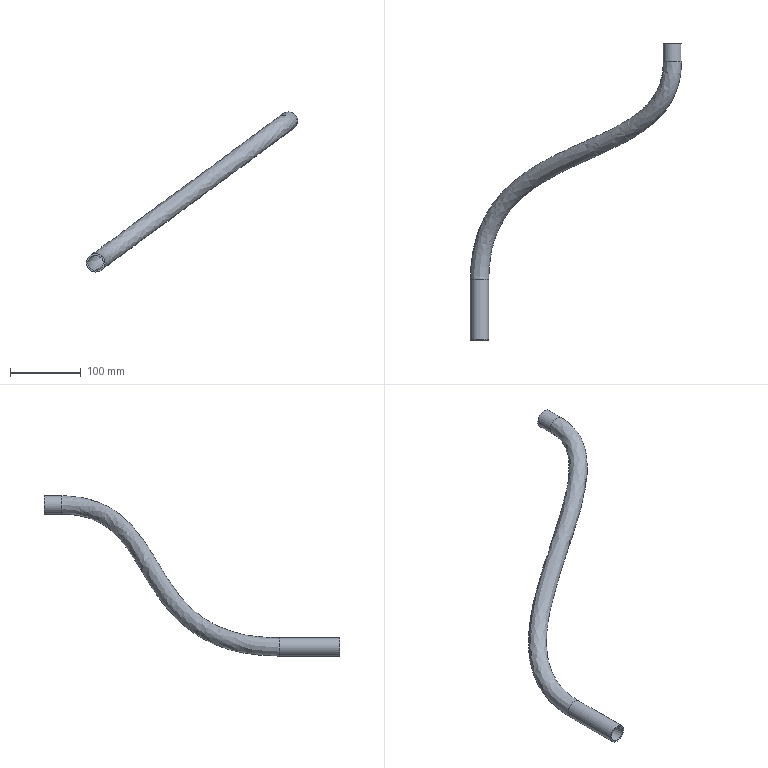Part | STEP file | Part 10^JBJ-F-0000-00 | 1 solid | 8 faces | box 298.36 x 417.992 x 226.424 mm | volume 91020 mm3 | cylinder 4 | spline 2 | plane 2 | commonest cylinder face diameters 22 x2 26 x2